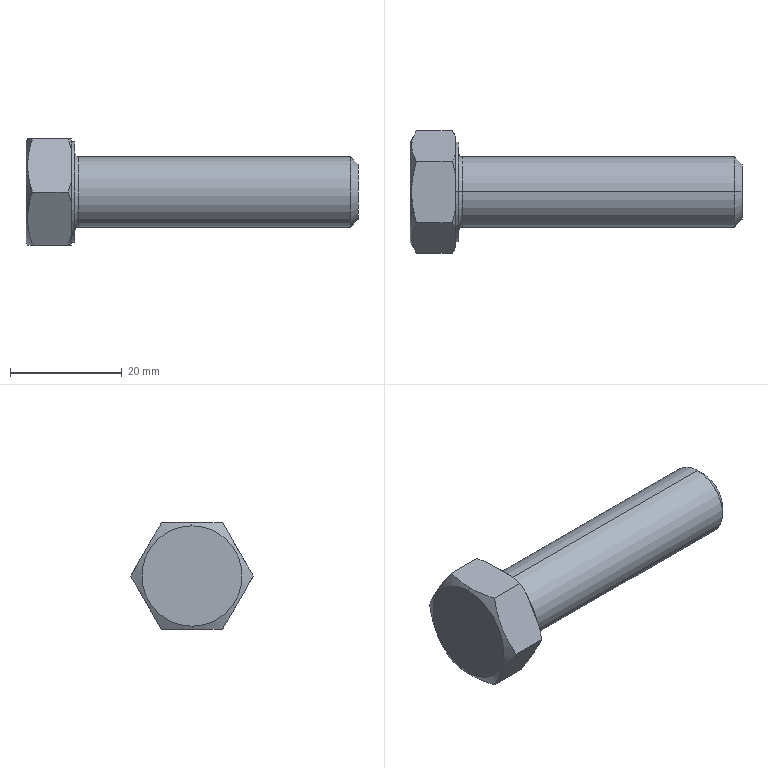Part | SolidWorks | features RevCut 4, Chamfer 1, Extrusion 1, Fillet 1, LPattern 1, Revolution 1 | 1 solid | 26 faces | box 59.531 x 21.997 x 19.05 mm | volume 9087 mm3 | cone 10 | plane 10 | cylinder 4 | torus 2 | commonest cylinder face diameters 12.7 x2 18 x2
STEP:
#1=CARTESIAN_POINT('',(9.331,0.,6.35));
#2=VERTEX_POINT('',#1);
#3=CARTESIAN_POINT('',(9.331,0.,-6.35));
#4=VERTEX_POINT('',#3);
#5=CARTESIAN_POINT('',(9.331,0.,0.));
#6=DIRECTION('',(1.,0.,0.));
#7=DIRECTION('',(0.,0.,-1.));
#8=AXIS2_PLACEMENT_3D('',#5,#6,#7);
#9=CIRCLE('',#8,6.35);
#10=EDGE_CURVE('',#2,#4,#9,.T.);
#11=ORIENTED_EDGE('',*,*,#10,.F.);
#12=CARTESIAN_POINT('',(8.731,0.,6.95));
#13=VERTEX_POINT('',#12);
#14=CARTESIAN_POINT('',(9.331,0.,6.95));
#15=DIRECTION('',(0.,1.,0.));
#16=DIRECTION('',(0.,0.,1.));
#17=AXIS2_PLACEMENT_3D('',#14,#15,#16);
#18=CIRCLE('',#17,0.6);
#19=EDGE_CURVE('',#2,#13,#18,.T.);
#20=ORIENTED_EDGE('',*,*,#19,.T.);
#21=CARTESIAN_POINT('',(8.731,0.,-6.95));
#22=VERTEX_POINT('',#21);
#23=CARTESIAN_POINT('',(8.731,0.,0.));
#24=DIRECTION('',(-1.,0.,0.));
#25=DIRECTION('',(0.,0.,-1.));
#26=AXIS2_PLACEMENT_3D('',#23,#24,#25);
#27=CIRCLE('',#26,6.95);
#28=EDGE_CURVE('',#22,#13,#27,.T.);
#29=ORIENTED_EDGE('',*,*,#28,.F.);
#30=CARTESIAN_POINT('',(9.331,0.,-6.95));
#31=DIRECTION('',(0.,-1.,0.));
#32=DIRECTION('',(0.,0.,-1.));
#33=AXIS2_PLACEMENT_3D('',#30,#31,#32);
#34=CIRCLE('',#33,0.6);
#35=EDGE_CURVE('',#4,#22,#34,.T.);
#36=ORIENTED_EDGE('',*,*,#35,.F.);
#37=EDGE_LOOP('',(#11,#20,#29,#36));
#38=FACE_OUTER_BOUND('',#37,.T.);
#39=CARTESIAN_POINT('',(9.331,0.,0.));
#40=DIRECTION('',(1.,0.,0.));
#41=DIRECTION('',(0.,0.,-1.));
#42=AXIS2_PLACEMENT_3D('',#39,#40,#41);
#43=TOROIDAL_SURFACE('',#42,6.95,0.6);
#44=ADVANCED_FACE('',(#38),#43,.F.);
#45=CARTESIAN_POINT('',(59.531,0.,-4.95));
#46=VERTEX_POINT('',#45);
#47=CARTESIAN_POINT('',(59.531,0.,4.95));
#48=VERTEX_POINT('',#47);
#49=CARTESIAN_POINT('',(59.531,0.,0.));
#50=DIRECTION('',(1.,0.,0.));
#51=DIRECTION('',(0.,0.,1.));
#52=AXIS2_PLACEMENT_3D('',#49,#50,#51);
#53=CIRCLE('',#52,4.95);
#54=EDGE_CURVE('',#46,#48,#53,.T.);
#55=ORIENTED_EDGE('',*,*,#54,.F.);
#56=CARTESIAN_POINT('',(58.131,0.,-6.35));
#57=VERTEX_POINT('',#56);
#58=CARTESIAN_POINT('',(58.131,0.,-6.35));
#59=DIRECTION('',(-0.7071,0.,-0.7071));
#60=VECTOR('',#59,1000.);
#61=LINE('',#58,#60);
#62=EDGE_CURVE('',#46,#57,#61,.T.);
#63=ORIENTED_EDGE('',*,*,#62,.T.);
#64=CARTESIAN_POINT('',(58.131,0.,6.35));
#65=VERTEX_POINT('',#64);
#66=CARTESIAN_POINT('',(58.131,0.,0.));
#67=DIRECTION('',(-1.,0.,0.));
#68=DIRECTION('',(0.,0.,1.));
#69=AXIS2_PLACEMENT_3D('',#66,#67,#68);
#70=CIRCLE('',#69,6.35);
#71=EDGE_CURVE('',#65,#57,#70,.T.);
#72=ORIENTED_EDGE('',*,*,#71,.F.);
#73=CARTESIAN_POINT('',(58.131,0.,6.35));
#74=DIRECTION('',(-0.7071,0.,0.7071));
#75=VECTOR('',#74,1000.);
#76=LINE('',#73,#75);
#77=EDGE_CURVE('',#48,#65,#76,.T.);
#78=ORIENTED_EDGE('',*,*,#77,.F.);
#79=EDGE_LOOP('',(#55,#63,#72,#78));
#80=FACE_OUTER_BOUND('',#79,.T.);
#81=CARTESIAN_POINT('',(58.131,0.,0.));
#82=DIRECTION('',(-1.,0.,0.));
#83=DIRECTION('',(0.,0.,1.));
#84=AXIS2_PLACEMENT_3D('',#81,#82,#83);
#85=CONICAL_SURFACE('',#84,6.35,0.7854);
#86=ADVANCED_FACE('',(#80),#85,.T.);
#87=ORIENTED_EDGE('',*,*,#71,.T.);
#88=CARTESIAN_POINT('',(0.,0.,-6.35));
#89=DIRECTION('',(-1.,0.,0.));
#90=VECTOR('',#89,1000.);
#91=LINE('',#88,#90);
#92=EDGE_CURVE('',#57,#4,#91,.T.);
#93=ORIENTED_EDGE('',*,*,#92,.T.);
#94=CARTESIAN_POINT('',(9.331,0.,0.));
#95=DIRECTION('',(1.,0.,0.));
#96=DIRECTION('',(0.,0.,-1.));
#97=AXIS2_PLACEMENT_3D('',#94,#95,#96);
#98=CIRCLE('',#97,6.35);
#99=EDGE_CURVE('',#4,#2,#98,.T.);
#100=ORIENTED_EDGE('',*,*,#99,.T.);
#101=CARTESIAN_POINT('',(0.,0.,6.35));
#102=DIRECTION('',(-1.,0.,0.));
#103=VECTOR('',#102,1000.);
#104=LINE('',#101,#103);
#105=EDGE_CURVE('',#65,#2,#104,.T.);
#106=ORIENTED_EDGE('',*,*,#105,.F.);
#107=EDGE_LOOP('',(#87,#93,#100,#106));
#108=FACE_OUTER_BOUND('',#107,.T.);
#109=CARTESIAN_POINT('',(0.,0.,0.));
#110=DIRECTION('',(-1.,0.,0.));
#111=DIRECTION('',(0.,0.,1.));
#112=AXIS2_PLACEMENT_3D('',#109,#110,#111);
#113=CYLINDRICAL_SURFACE('',#112,6.35);
#114=ADVANCED_FACE('',(#108),#113,.T.);
#115=CARTESIAN_POINT('',(8.731,0.,9.));
#116=VERTEX_POINT('',#115);
#117=CARTESIAN_POINT('',(8.731,0.,-9.));
#118=VERTEX_POINT('',#117);
#119=CARTESIAN_POINT('',(8.731,0.,0.));
#120=DIRECTION('',(-1.,0.,0.));
#121=DIRECTION('',(0.,0.,1.));
#122=AXIS2_PLACEMENT_3D('',#119,#120,#121);
#123=CIRCLE('',#122,9.);
#124=EDGE_CURVE('',#116,#118,#123,.T.);
#125=ORIENTED_EDGE('',*,*,#124,.T.);
#126=CARTESIAN_POINT('',(8.131,0.,-9.));
#127=VERTEX_POINT('',#126);
#128=CARTESIAN_POINT('',(0.,0.,-9.));
#129=DIRECTION('',(-1.,0.,0.));
#130=VECTOR('',#129,1000.);
#131=LINE('',#128,#130);
#132=EDGE_CURVE('',#118,#127,#131,.T.);
#133=ORIENTED_EDGE('',*,*,#132,.T.);
#134=CARTESIAN_POINT('',(8.131,0.,9.));
#135=VERTEX_POINT('',#134);
#136=CARTESIAN_POINT('',(8.131,0.,0.));
#137=DIRECTION('',(-1.,0.,0.));
#138=DIRECTION('',(0.,0.,1.));
#139=AXIS2_PLACEMENT_3D('',#136,#137,#138);
#140=CIRCLE('',#139,9.);
#141=EDGE_CURVE('',#135,#127,#140,.T.);
#142=ORIENTED_EDGE('',*,*,#141,.F.);
#143=CARTESIAN_POINT('',(0.,0.,9.));
#144=DIRECTION('',(-1.,0.,0.));
#145=VECTOR('',#144,1000.);
#146=LINE('',#143,#145);
#147=EDGE_CURVE('',#116,#135,#146,.T.);
#148=ORIENTED_EDGE('',*,*,#147,.F.);
#149=EDGE_LOOP('',(#125,#133,#142,#148));
#150=FACE_OUTER_BOUND('',#149,.T.);
#151=CARTESIAN_POINT('',(0.,0.,0.));
#152=DIRECTION('',(-1.,0.,0.));
#153=DIRECTION('',(0.,0.,1.));
#154=AXIS2_PLACEMENT_3D('',#151,#152,#153);
#155=CYLINDRICAL_SURFACE('',#154,9.);
#156=ADVANCED_FACE('',(#150),#155,.T.);
#157=CARTESIAN_POINT('',(0.,0.,9.));
#158=VERTEX_POINT('',#157);
#159=CARTESIAN_POINT('',(0.,0.,-9.));
#160=VERTEX_POINT('',#159);
#161=CARTESIAN_POINT('',(0.,0.,0.));
#162=DIRECTION('',(-1.,0.,0.));
#163=DIRECTION('',(0.,0.,1.));
#164=AXIS2_PLACEMENT_3D('',#161,#162,#163);
#165=CIRCLE('',#164,9.);
#166=EDGE_CURVE('',#158,#160,#165,.T.);
#167=ORIENTED_EDGE('',*,*,#166,.F.);
#168=CARTESIAN_POINT('',(0.3031,0.,9.525));
#169=VERTEX_POINT('',#168);
#170=CARTESIAN_POINT('',(0.,0.,9.));
#171=DIRECTION('',(0.5,0.,0.866));
#172=VECTOR('',#171,1000.);
#173=LINE('',#170,#172);
#174=EDGE_CURVE('',#158,#169,#173,.T.);
#175=ORIENTED_EDGE('',*,*,#174,.T.);
#176=CARTESIAN_POINT('',(1.154,5.499,9.525));
#177=VERTEX_POINT('',#176);
#178=CARTESIAN_POINT('',(0.3031,0.,9.525));
#179=CARTESIAN_POINT('',(0.3031,0.4656,9.525));
#180=CARTESIAN_POINT('',(0.323,0.9341,9.525));
#181=CARTESIAN_POINT('',(0.4017,1.87,9.525));
#182=CARTESIAN_POINT('',(0.4599,2.333,9.525));
#183=CARTESIAN_POINT('',(0.6834,3.709,9.525));
#184=CARTESIAN_POINT('',(0.8971,4.61,9.525));
#185=CARTESIAN_POINT('',(1.154,5.499,9.525));
#186=B_SPLINE_CURVE_WITH_KNOTS('',3,(#178,#179,#180,#181,#182,#183,#184,#185),.UNSPECIFIED.,.F.,.F.,(4,2,2,4),(0.01578,0.01717,0.01857,0.02135),.UNSPECIFIED.);
#187=EDGE_CURVE('',#169,#177,#186,.T.);
#188=ORIENTED_EDGE('',*,*,#187,.T.);
#189=CARTESIAN_POINT('',(1.154,10.999,0.));
#190=VERTEX_POINT('',#189);
#191=CARTESIAN_POINT('',(1.154,5.499,9.525));
#192=CARTESIAN_POINT('',(0.8946,5.948,8.747));
#193=CARTESIAN_POINT('',(0.681,6.4,7.964));
#194=CARTESIAN_POINT('',(0.3851,7.314,6.381));
#195=CARTESIAN_POINT('',(0.3037,7.776,5.581));
#196=CARTESIAN_POINT('',(0.3028,8.477,4.367));
#197=CARTESIAN_POINT('',(0.3227,8.712,3.96));
#198=CARTESIAN_POINT('',(0.4002,9.177,3.155));
#199=CARTESIAN_POINT('',(0.4578,9.408,2.756));
#200=CARTESIAN_POINT('',(0.6802,10.096,1.564));
#201=CARTESIAN_POINT('',(0.8943,10.549,0.7786));
#202=CARTESIAN_POINT('',(1.154,10.999,0.));
#203=B_SPLINE_CURVE_WITH_KNOTS('',3,(#191,#192,#193,#194,#195,#196,#197,#198,#199,#200,#201,#202),.UNSPECIFIED.,.F.,.F.,(4,2,2,2,2,4),(0.000000238,0.002777,0.005554,0.006943,0.008331,0.01111),.UNSPECIFIED.);
#204=EDGE_CURVE('',#177,#190,#203,.T.);
#205=ORIENTED_EDGE('',*,*,#204,.T.);
#206=CARTESIAN_POINT('',(1.154,5.499,-9.525));
#207=VERTEX_POINT('',#206);
#208=CARTESIAN_POINT('',(1.154,10.999,0.));
#209=CARTESIAN_POINT('',(0.8946,10.55,-0.7776));
#210=CARTESIAN_POINT('',(0.681,10.097,-1.561));
#211=CARTESIAN_POINT('',(0.3851,9.183,-3.144));
#212=CARTESIAN_POINT('',(0.3037,8.722,-3.944));
#213=CARTESIAN_POINT('',(0.3028,8.02,-5.158));
#214=CARTESIAN_POINT('',(0.3227,7.786,-5.565));
#215=CARTESIAN_POINT('',(0.4002,7.321,-6.37));
#216=CARTESIAN_POINT('',(0.4578,7.09,-6.769));
#217=CARTESIAN_POINT('',(0.6802,6.402,-7.961));
#218=CARTESIAN_POINT('',(0.8943,5.949,-8.746));
#219=CARTESIAN_POINT('',(1.154,5.499,-9.525));
#220=B_SPLINE_CURVE_WITH_KNOTS('',3,(#208,#209,#210,#211,#212,#213,#214,#215,#216,#217,#218,#219),.UNSPECIFIED.,.F.,.F.,(4,2,2,2,2,4),(0.000000238,0.002777,0.005554,0.006943,0.008331,0.01111),.UNSPECIFIED.);
#221=EDGE_CURVE('',#190,#207,#220,.T.);
#222=ORIENTED_EDGE('',*,*,#221,.T.);
#223=CARTESIAN_POINT('',(0.3031,0.,-9.525));
#224=VERTEX_POINT('',#223);
#225=CARTESIAN_POINT('',(1.154,5.499,-9.525));
#226=CARTESIAN_POINT('',(0.8971,4.61,-9.525));
#227=CARTESIAN_POINT('',(0.6834,3.709,-9.525));
#228=CARTESIAN_POINT('',(0.4599,2.333,-9.525));
#229=CARTESIAN_POINT('',(0.4017,1.87,-9.525));
#230=CARTESIAN_POINT('',(0.323,0.9341,-9.525));
#231=CARTESIAN_POINT('',(0.3031,0.4656,-9.525));
#232=CARTESIAN_POINT('',(0.3031,0.,-9.525));
#233=B_SPLINE_CURVE_WITH_KNOTS('',3,(#225,#226,#227,#228,#229,#230,#231,#232),.UNSPECIFIED.,.F.,.F.,(4,2,2,4),(0.02694,0.02972,0.03112,0.03251),.UNSPECIFIED.);
#234=EDGE_CURVE('',#207,#224,#233,.T.);
#235=ORIENTED_EDGE('',*,*,#234,.T.);
#236=CARTESIAN_POINT('',(0.,0.,-9.));
#237=DIRECTION('',(0.5,0.,-0.866));
#238=VECTOR('',#237,1000.);
#239=LINE('',#236,#238);
#240=EDGE_CURVE('',#160,#224,#239,.T.);
#241=ORIENTED_EDGE('',*,*,#240,.F.);
#242=EDGE_LOOP('',(#167,#175,#188,#205,#222,#235,#241));
#243=FACE_OUTER_BOUND('',#242,.T.);
#244=CARTESIAN_POINT('',(0.,0.,0.));
#245=DIRECTION('',(1.,0.,0.));
#246=DIRECTION('',(0.,0.,-1.));
#247=AXIS2_PLACEMENT_3D('',#244,#245,#246);
#248=CONICAL_SURFACE('',#247,9.,1.047);
#249=ADVANCED_FACE('',(#243),#248,.T.);
#250=CARTESIAN_POINT('',(8.131,6.663,-7.509));
#251=VERTEX_POINT('',#250);
#252=CARTESIAN_POINT('',(8.131,9.835,-2.016));
#253=VERTEX_POINT('',#252);
#254=CARTESIAN_POINT('',(8.131,5.499,-9.525));
#255=DIRECTION('',(0.,0.5,0.866));
#256=VECTOR('',#255,1000.);
#257=LINE('',#254,#256);
#258=EDGE_CURVE('',#251,#253,#257,.T.);
#259=ORIENTED_EDGE('',*,*,#258,.F.);
#260=CARTESIAN_POINT('',(7.577,5.499,-9.525));
#261=VERTEX_POINT('',#260);
#262=CARTESIAN_POINT('',(7.577,5.499,-9.525));
#263=CARTESIAN_POINT('',(7.8,5.884,-8.858));
#264=CARTESIAN_POINT('',(7.989,6.272,-8.186));
#265=CARTESIAN_POINT('',(8.131,6.663,-7.509));
#266=B_SPLINE_CURVE_WITH_KNOTS('',3,(#262,#263,#264,#265),.UNSPECIFIED.,.F.,.F.,(4,4),(0.000000238,0.002383),.UNSPECIFIED.);
#267=EDGE_CURVE('',#261,#251,#266,.T.);
#268=ORIENTED_EDGE('',*,*,#267,.F.);
#269=CARTESIAN_POINT('',(8.731,5.499,-9.525));
#270=DIRECTION('',(-1.,0.,0.));
#271=VECTOR('',#270,1000.);
#272=LINE('',#269,#271);
#273=EDGE_CURVE('',#261,#207,#272,.T.);
#274=ORIENTED_EDGE('',*,*,#273,.T.);
#275=ORIENTED_EDGE('',*,*,#221,.F.);
#276=CARTESIAN_POINT('',(7.577,10.999,0.));
#277=VERTEX_POINT('',#276);
#278=CARTESIAN_POINT('',(8.731,10.999,0.));
#279=DIRECTION('',(-1.,0.,0.));
#280=VECTOR('',#279,1000.);
#281=LINE('',#278,#280);
#282=EDGE_CURVE('',#277,#190,#281,.T.);
#283=ORIENTED_EDGE('',*,*,#282,.F.);
#284=CARTESIAN_POINT('',(8.131,9.835,-2.016));
#285=CARTESIAN_POINT('',(7.988,10.226,-1.338));
#286=CARTESIAN_POINT('',(7.8,10.614,-0.6665));
#287=CARTESIAN_POINT('',(7.577,10.999,0.));
#288=B_SPLINE_CURVE_WITH_KNOTS('',3,(#284,#285,#286,#287),.UNSPECIFIED.,.F.,.F.,(4,4),(0.008731,0.01111),.UNSPECIFIED.);
#289=EDGE_CURVE('',#253,#277,#288,.T.);
#290=ORIENTED_EDGE('',*,*,#289,.F.);
#291=EDGE_LOOP('',(#259,#268,#274,#275,#283,#290));
#292=FACE_OUTER_BOUND('',#291,.T.);
#293=CARTESIAN_POINT('',(8.731,5.499,-9.525));
#294=DIRECTION('',(0.,-0.866,0.5));
#295=DIRECTION('',(0.,-0.5,-0.866));
#296=AXIS2_PLACEMENT_3D('',#293,#294,#295);
#297=PLANE('',#296);
#298=ADVANCED_FACE('',(#292),#297,.F.);
#299=CARTESIAN_POINT('',(8.131,9.835,2.016));
#300=VERTEX_POINT('',#299);
#301=CARTESIAN_POINT('',(8.131,6.663,7.509));
#302=VERTEX_POINT('',#301);
#303=CARTESIAN_POINT('',(8.131,10.999,0.));
#304=DIRECTION('',(0.,-0.5,0.866));
#305=VECTOR('',#304,1000.);
#306=LINE('',#303,#305);
#307=EDGE_CURVE('',#300,#302,#306,.T.);
#308=ORIENTED_EDGE('',*,*,#307,.F.);
#309=CARTESIAN_POINT('',(7.577,10.999,0.));
#310=CARTESIAN_POINT('',(7.8,10.613,0.6672));
#311=CARTESIAN_POINT('',(7.989,10.226,1.339));
#312=CARTESIAN_POINT('',(8.131,9.835,2.016));
#313=B_SPLINE_CURVE_WITH_KNOTS('',3,(#309,#310,#311,#312),.UNSPECIFIED.,.F.,.F.,(4,4),(0.000000238,0.002383),.UNSPECIFIED.);
#314=EDGE_CURVE('',#277,#300,#313,.T.);
#315=ORIENTED_EDGE('',*,*,#314,.F.);
#316=ORIENTED_EDGE('',*,*,#282,.T.);
#317=ORIENTED_EDGE('',*,*,#204,.F.);
#318=CARTESIAN_POINT('',(7.577,5.499,9.525));
#319=VERTEX_POINT('',#318);
#320=CARTESIAN_POINT('',(8.731,5.499,9.525));
#321=DIRECTION('',(-1.,0.,0.));
#322=VECTOR('',#321,1000.);
#323=LINE('',#320,#322);
#324=EDGE_CURVE('',#319,#177,#323,.T.);
#325=ORIENTED_EDGE('',*,*,#324,.F.);
#326=CARTESIAN_POINT('',(8.131,6.663,7.509));
#327=CARTESIAN_POINT('',(7.988,6.272,8.187));
#328=CARTESIAN_POINT('',(7.8,5.884,8.859));
#329=CARTESIAN_POINT('',(7.577,5.499,9.525));
#330=B_SPLINE_CURVE_WITH_KNOTS('',3,(#326,#327,#328,#329),.UNSPECIFIED.,.F.,.F.,(4,4),(0.008731,0.01111),.UNSPECIFIED.);
#331=EDGE_CURVE('',#302,#319,#330,.T.);
#332=ORIENTED_EDGE('',*,*,#331,.F.);
#333=EDGE_LOOP('',(#308,#315,#316,#317,#325,#332));
#334=FACE_OUTER_BOUND('',#333,.T.);
#335=CARTESIAN_POINT('',(8.731,10.999,0.));
#336=DIRECTION('',(0.,-0.866,-0.5));
#337=DIRECTION('',(0.,0.5,-0.866));
#338=AXIS2_PLACEMENT_3D('',#335,#336,#337);
#339=PLANE('',#338);
#340=ADVANCED_FACE('',(#334),#339,.F.);
#341=CARTESIAN_POINT('',(8.131,3.172,9.525));
#342=VERTEX_POINT('',#341);
#343=CARTESIAN_POINT('',(8.131,-3.172,9.525));
#344=VERTEX_POINT('',#343);
#345=CARTESIAN_POINT('',(8.131,5.499,9.525));
#346=DIRECTION('',(0.,-1.,0.));
#347=VECTOR('',#346,1000.);
#348=LINE('',#345,#347);
#349=EDGE_CURVE('',#342,#344,#348,.T.);
#350=ORIENTED_EDGE('',*,*,#349,.F.);
#351=CARTESIAN_POINT('',(7.577,5.499,9.525));
#352=CARTESIAN_POINT('',(7.799,4.733,9.525));
#353=CARTESIAN_POINT('',(7.988,3.958,9.525));
#354=CARTESIAN_POINT('',(8.131,3.172,9.525));
#355=B_SPLINE_CURVE_WITH_KNOTS('',3,(#351,#352,#353,#354),.UNSPECIFIED.,.F.,.F.,(4,4),(0.02694,0.02934),.UNSPECIFIED.);
#356=EDGE_CURVE('',#319,#342,#355,.T.);
#357=ORIENTED_EDGE('',*,*,#356,.F.);
#358=ORIENTED_EDGE('',*,*,#324,.T.);
#359=ORIENTED_EDGE('',*,*,#187,.F.);
#360=CARTESIAN_POINT('',(1.154,-5.499,9.525));
#361=VERTEX_POINT('',#360);
#362=CARTESIAN_POINT('',(1.154,-5.499,9.525));
#363=CARTESIAN_POINT('',(0.8953,-4.604,9.525));
#364=CARTESIAN_POINT('',(0.679,-3.688,9.525));
#365=CARTESIAN_POINT('',(0.3832,-1.854,9.525));
#366=CARTESIAN_POINT('',(0.3031,-0.9305,9.525));
#367=CARTESIAN_POINT('',(0.3031,0.,9.525));
#368=B_SPLINE_CURVE_WITH_KNOTS('',3,(#362,#363,#364,#365,#366,#367),.UNSPECIFIED.,.F.,.F.,(4,2,4),(0.01021,0.013,0.01578),.UNSPECIFIED.);
#369=EDGE_CURVE('',#361,#169,#368,.T.);
#370=ORIENTED_EDGE('',*,*,#369,.F.);
#371=CARTESIAN_POINT('',(7.577,-5.499,9.525));
#372=VERTEX_POINT('',#371);
#373=CARTESIAN_POINT('',(8.731,-5.499,9.525));
#374=DIRECTION('',(-1.,0.,0.));
#375=VECTOR('',#374,1000.);
#376=LINE('',#373,#375);
#377=EDGE_CURVE('',#372,#361,#376,.T.);
#378=ORIENTED_EDGE('',*,*,#377,.F.);
#379=CARTESIAN_POINT('',(8.131,-3.172,9.525));
#380=CARTESIAN_POINT('',(7.989,-3.954,9.525));
#381=CARTESIAN_POINT('',(7.798,-4.734,9.525));
#382=CARTESIAN_POINT('',(7.577,-5.499,9.525));
#383=B_SPLINE_CURVE_WITH_KNOTS('',3,(#379,#380,#381,#382),.UNSPECIFIED.,.F.,.F.,(4,4),(0.0357,0.03808),.UNSPECIFIED.);
#384=EDGE_CURVE('',#344,#372,#383,.T.);
#385=ORIENTED_EDGE('',*,*,#384,.F.);
#386=EDGE_LOOP('',(#350,#357,#358,#359,#370,#378,#385));
#387=FACE_OUTER_BOUND('',#386,.T.);
#388=CARTESIAN_POINT('',(8.731,5.499,9.525));
#389=DIRECTION('',(0.,0.,-1.));
#390=DIRECTION('',(-1.,0.,0.));
#391=AXIS2_PLACEMENT_3D('',#388,#389,#390);
#392=PLANE('',#391);
#393=ADVANCED_FACE('',(#387),#392,.F.);
#394=CARTESIAN_POINT('',(8.131,-6.663,7.509));
#395=VERTEX_POINT('',#394);
#396=CARTESIAN_POINT('',(8.131,-9.835,2.016));
#397=VERTEX_POINT('',#396);
#398=CARTESIAN_POINT('',(8.131,-10.999,0.));
#399=DIRECTION('',(0.,-0.5,-0.866));
#400=VECTOR('',#399,1000.);
#401=LINE('',#398,#400);
#402=EDGE_CURVE('',#395,#397,#401,.T.);
#403=ORIENTED_EDGE('',*,*,#402,.F.);
#404=CARTESIAN_POINT('',(7.577,-5.499,9.525));
#405=CARTESIAN_POINT('',(7.8,-5.884,8.858));
#406=CARTESIAN_POINT('',(7.989,-6.272,8.186));
#407=CARTESIAN_POINT('',(8.131,-6.663,7.509));
#408=B_SPLINE_CURVE_WITH_KNOTS('',3,(#404,#405,#406,#407),.UNSPECIFIED.,.F.,.F.,(4,4),(0.000000238,0.002383),.UNSPECIFIED.);
#409=EDGE_CURVE('',#372,#395,#408,.T.);
#410=ORIENTED_EDGE('',*,*,#409,.F.);
#411=ORIENTED_EDGE('',*,*,#377,.T.);
#412=CARTESIAN_POINT('',(1.154,-10.999,0.));
#413=VERTEX_POINT('',#412);
#414=CARTESIAN_POINT('',(1.154,-10.999,0.));
#415=CARTESIAN_POINT('',(0.8946,-10.55,0.7776));
#416=CARTESIAN_POINT('',(0.681,-10.097,1.561));
#417=CARTESIAN_POINT('',(0.3851,-9.183,3.144));
#418=CARTESIAN_POINT('',(0.3037,-8.722,3.944));
#419=CARTESIAN_POINT('',(0.3028,-8.02,5.158));
#420=CARTESIAN_POINT('',(0.3227,-7.786,5.565));
#421=CARTESIAN_POINT('',(0.4002,-7.321,6.37));
#422=CARTESIAN_POINT('',(0.4578,-7.09,6.769));
#423=CARTESIAN_POINT('',(0.6802,-6.402,7.961));
#424=CARTESIAN_POINT('',(0.8943,-5.949,8.746));
#425=CARTESIAN_POINT('',(1.154,-5.499,9.525));
#426=B_SPLINE_CURVE_WITH_KNOTS('',3,(#414,#415,#416,#417,#418,#419,#420,#421,#422,#423,#424,#425),.UNSPECIFIED.,.F.,.F.,(4,2,2,2,2,4),(0.000000238,0.002777,0.005554,0.006943,0.008331,0.01111),.UNSPECIFIED.);
#427=EDGE_CURVE('',#413,#361,#426,.T.);
#428=ORIENTED_EDGE('',*,*,#427,.F.);
#429=CARTESIAN_POINT('',(7.577,-10.999,0.));
#430=VERTEX_POINT('',#429);
#431=CARTESIAN_POINT('',(8.731,-10.999,0.));
#432=DIRECTION('',(-1.,0.,0.));
#433=VECTOR('',#432,1000.);
#434=LINE('',#431,#433);
#435=EDGE_CURVE('',#430,#413,#434,.T.);
#436=ORIENTED_EDGE('',*,*,#435,.F.);
#437=CARTESIAN_POINT('',(8.131,-9.835,2.016));
#438=CARTESIAN_POINT('',(7.988,-10.226,1.338));
#439=CARTESIAN_POINT('',(7.8,-10.614,0.6665));
#440=CARTESIAN_POINT('',(7.577,-10.999,0.));
#441=B_SPLINE_CURVE_WITH_KNOTS('',3,(#437,#438,#439,#440),.UNSPECIFIED.,.F.,.F.,(4,4),(0.008731,0.01111),.UNSPECIFIED.);
#442=EDGE_CURVE('',#397,#430,#441,.T.);
#443=ORIENTED_EDGE('',*,*,#442,.F.);
#444=EDGE_LOOP('',(#403,#410,#411,#428,#436,#443));
#445=FACE_OUTER_BOUND('',#444,.T.);
#446=CARTESIAN_POINT('',(8.731,-10.999,0.));
#447=DIRECTION('',(0.,0.866,-0.5));
#448=DIRECTION('',(0.,0.5,0.866));
#449=AXIS2_PLACEMENT_3D('',#446,#447,#448);
#450=PLANE('',#449);
#451=ADVANCED_FACE('',(#445),#450,.F.);
#452=CARTESIAN_POINT('',(8.131,-9.835,-2.016));
#453=VERTEX_POINT('',#452);
#454=CARTESIAN_POINT('',(8.131,-6.663,-7.509));
#455=VERTEX_POINT('',#454);
#456=CARTESIAN_POINT('',(8.131,-5.499,-9.525));
#457=DIRECTION('',(0.,0.5,-0.866));
#458=VECTOR('',#457,1000.);
#459=LINE('',#456,#458);
#460=EDGE_CURVE('',#453,#455,#459,.T.);
#461=ORIENTED_EDGE('',*,*,#460,.F.);
#462=CARTESIAN_POINT('',(7.577,-10.999,0.));
#463=CARTESIAN_POINT('',(7.8,-10.613,-0.6672));
#464=CARTESIAN_POINT('',(7.989,-10.226,-1.339));
#465=CARTESIAN_POINT('',(8.131,-9.835,-2.016));
#466=B_SPLINE_CURVE_WITH_KNOTS('',3,(#462,#463,#464,#465),.UNSPECIFIED.,.F.,.F.,(4,4),(0.000000238,0.002383),.UNSPECIFIED.);
#467=EDGE_CURVE('',#430,#453,#466,.T.);
#468=ORIENTED_EDGE('',*,*,#467,.F.);
#469=ORIENTED_EDGE('',*,*,#435,.T.);
#470=CARTESIAN_POINT('',(1.154,-5.499,-9.525));
#471=VERTEX_POINT('',#470);
#472=CARTESIAN_POINT('',(1.154,-5.499,-9.525));
#473=CARTESIAN_POINT('',(0.8946,-5.948,-8.747));
#474=CARTESIAN_POINT('',(0.681,-6.4,-7.964));
#475=CARTESIAN_POINT('',(0.3851,-7.314,-6.381));
#476=CARTESIAN_POINT('',(0.3037,-7.776,-5.581));
#477=CARTESIAN_POINT('',(0.3028,-8.477,-4.367));
#478=CARTESIAN_POINT('',(0.3227,-8.712,-3.96));
#479=CARTESIAN_POINT('',(0.4002,-9.177,-3.155));
#480=CARTESIAN_POINT('',(0.4578,-9.408,-2.756));
#481=CARTESIAN_POINT('',(0.6802,-10.096,-1.564));
#482=CARTESIAN_POINT('',(0.8943,-10.549,-0.7786));
#483=CARTESIAN_POINT('',(1.154,-10.999,0.));
#484=B_SPLINE_CURVE_WITH_KNOTS('',3,(#472,#473,#474,#475,#476,#477,#478,#479,#480,#481,#482,#483),.UNSPECIFIED.,.F.,.F.,(4,2,2,2,2,4),(0.000000238,0.002777,0.005554,0.006943,0.008331,0.01111),.UNSPECIFIED.);
#485=EDGE_CURVE('',#471,#413,#484,.T.);
#486=ORIENTED_EDGE('',*,*,#485,.F.);
#487=CARTESIAN_POINT('',(7.577,-5.499,-9.525));
#488=VERTEX_POINT('',#487);
#489=CARTESIAN_POINT('',(8.731,-5.499,-9.525));
#490=DIRECTION('',(-1.,0.,0.));
#491=VECTOR('',#490,1000.);
#492=LINE('',#489,#491);
#493=EDGE_CURVE('',#488,#471,#492,.T.);
#494=ORIENTED_EDGE('',*,*,#493,.F.);
#495=CARTESIAN_POINT('',(8.131,-6.663,-7.509));
#496=CARTESIAN_POINT('',(7.988,-6.272,-8.187));
#497=CARTESIAN_POINT('',(7.8,-5.884,-8.859));
#498=CARTESIAN_POINT('',(7.577,-5.499,-9.525));
#499=B_SPLINE_CURVE_WITH_KNOTS('',3,(#495,#496,#497,#498),.UNSPECIFIED.,.F.,.F.,(4,4),(0.008731,0.01111),.UNSPECIFIED.);
#500=EDGE_CURVE('',#455,#488,#499,.T.);
#501=ORIENTED_EDGE('',*,*,#500,.F.);
#502=EDGE_LOOP('',(#461,#468,#469,#486,#494,#501));
#503=FACE_OUTER_BOUND('',#502,.T.);
#504=CARTESIAN_POINT('',(8.731,-5.499,-9.525));
#505=DIRECTION('',(0.,0.866,0.5));
#506=DIRECTION('',(0.,-0.5,0.866));
#507=AXIS2_PLACEMENT_3D('',#504,#505,#506);
#508=PLANE('',#507);
#509=ADVANCED_FACE('',(#503),#508,.F.);
#510=CARTESIAN_POINT('',(8.131,-3.172,-9.525));
#511=VERTEX_POINT('',#510);
#512=CARTESIAN_POINT('',(8.131,3.172,-9.525));
#513=VERTEX_POINT('',#512);
#514=CARTESIAN_POINT('',(8.131,5.499,-9.525));
#515=DIRECTION('',(0.,1.,0.));
#516=VECTOR('',#515,1000.);
#517=LINE('',#514,#516);
#518=EDGE_CURVE('',#511,#513,#517,.T.);
#519=ORIENTED_EDGE('',*,*,#518,.F.);
#520=CARTESIAN_POINT('',(7.577,-5.499,-9.525));
#521=CARTESIAN_POINT('',(7.798,-4.734,-9.525));
#522=CARTESIAN_POINT('',(7.989,-3.954,-9.525));
#523=CARTESIAN_POINT('',(8.131,-3.172,-9.525));
#524=B_SPLINE_CURVE_WITH_KNOTS('',3,(#520,#521,#522,#523),.UNSPECIFIED.,.F.,.F.,(4,4),(0.01021,0.01259),.UNSPECIFIED.);
#525=EDGE_CURVE('',#488,#511,#524,.T.);
#526=ORIENTED_EDGE('',*,*,#525,.F.);
#527=ORIENTED_EDGE('',*,*,#493,.T.);
#528=CARTESIAN_POINT('',(0.3031,0.,-9.525));
#529=CARTESIAN_POINT('',(0.3031,-0.9305,-9.525));
#530=CARTESIAN_POINT('',(0.3832,-1.854,-9.525));
#531=CARTESIAN_POINT('',(0.679,-3.688,-9.525));
#532=CARTESIAN_POINT('',(0.8953,-4.604,-9.525));
#533=CARTESIAN_POINT('',(1.154,-5.499,-9.525));
#534=B_SPLINE_CURVE_WITH_KNOTS('',3,(#528,#529,#530,#531,#532,#533),.UNSPECIFIED.,.F.,.F.,(4,2,4),(0.03251,0.03529,0.03808),.UNSPECIFIED.);
#535=EDGE_CURVE('',#224,#471,#534,.T.);
#536=ORIENTED_EDGE('',*,*,#535,.F.);
#537=ORIENTED_EDGE('',*,*,#234,.F.);
#538=ORIENTED_EDGE('',*,*,#273,.F.);
#539=CARTESIAN_POINT('',(8.131,3.172,-9.525));
#540=CARTESIAN_POINT('',(7.988,3.958,-9.525));
#541=CARTESIAN_POINT('',(7.799,4.733,-9.525));
#542=CARTESIAN_POINT('',(7.577,5.499,-9.525));
#543=B_SPLINE_CURVE_WITH_KNOTS('',3,(#539,#540,#541,#542),.UNSPECIFIED.,.F.,.F.,(4,4),(0.01895,0.02135),.UNSPECIFIED.);
#544=EDGE_CURVE('',#513,#261,#543,.T.);
#545=ORIENTED_EDGE('',*,*,#544,.F.);
#546=EDGE_LOOP('',(#519,#526,#527,#536,#537,#538,#545));
#547=FACE_OUTER_BOUND('',#546,.T.);
#548=CARTESIAN_POINT('',(8.731,5.499,-9.525));
#549=DIRECTION('',(0.,0.,1.));
#550=DIRECTION('',(1.,0.,0.));
#551=AXIS2_PLACEMENT_3D('',#548,#549,#550);
#552=PLANE('',#551);
#553=ADVANCED_FACE('',(#547),#552,.F.);
#554=ORIENTED_EDGE('',*,*,#525,.T.);
#555=CARTESIAN_POINT('',(8.131,0.,0.));
#556=DIRECTION('',(-1.,0.,0.));
#557=DIRECTION('',(0.,0.,-1.));
#558=AXIS2_PLACEMENT_3D('',#555,#556,#557);
#559=CIRCLE('',#558,10.039);
#560=EDGE_CURVE('',#511,#455,#559,.T.);
#561=ORIENTED_EDGE('',*,*,#560,.T.);
#562=ORIENTED_EDGE('',*,*,#500,.T.);
#563=EDGE_LOOP('',(#554,#561,#562));
#564=FACE_OUTER_BOUND('',#563,.T.);
#565=CARTESIAN_POINT('',(4.691,0.,0.));
#566=DIRECTION('',(-1.,0.,0.));
#567=DIRECTION('',(0.,0.,1.));
#568=AXIS2_PLACEMENT_3D('',#565,#566,#567);
#569=CONICAL_SURFACE('',#568,15.999,1.047);
#570=ADVANCED_FACE('',(#564),#569,.T.);
#571=ORIENTED_EDGE('',*,*,#467,.T.);
#572=CARTESIAN_POINT('',(8.131,0.,0.));
#573=DIRECTION('',(-1.,0.,0.));
#574=DIRECTION('',(0.,0.,-1.));
#575=AXIS2_PLACEMENT_3D('',#572,#573,#574);
#576=CIRCLE('',#575,10.039);
#577=EDGE_CURVE('',#453,#397,#576,.T.);
#578=ORIENTED_EDGE('',*,*,#577,.T.);
#579=ORIENTED_EDGE('',*,*,#442,.T.);
#580=EDGE_LOOP('',(#571,#578,#579));
#581=FACE_OUTER_BOUND('',#580,.T.);
#582=CARTESIAN_POINT('',(4.691,0.,0.));
#583=DIRECTION('',(-1.,0.,0.));
#584=DIRECTION('',(0.,0.,1.));
#585=AXIS2_PLACEMENT_3D('',#582,#583,#584);
#586=CONICAL_SURFACE('',#585,15.999,1.047);
#587=ADVANCED_FACE('',(#581),#586,.T.);
#588=ORIENTED_EDGE('',*,*,#409,.T.);
#589=CARTESIAN_POINT('',(8.131,0.,0.));
#590=DIRECTION('',(-1.,0.,0.));
#591=DIRECTION('',(0.,0.,-1.));
#592=AXIS2_PLACEMENT_3D('',#589,#590,#591);
#593=CIRCLE('',#592,10.039);
#594=EDGE_CURVE('',#395,#344,#593,.T.);
#595=ORIENTED_EDGE('',*,*,#594,.T.);
#596=ORIENTED_EDGE('',*,*,#384,.T.);
#597=EDGE_LOOP('',(#588,#595,#596));
#598=FACE_OUTER_BOUND('',#597,.T.);
#599=CARTESIAN_POINT('',(4.691,0.,0.));
#600=DIRECTION('',(-1.,0.,0.));
#601=DIRECTION('',(0.,0.,1.));
#602=AXIS2_PLACEMENT_3D('',#599,#600,#601);
#603=CONICAL_SURFACE('',#602,15.999,1.047);
#604=ADVANCED_FACE('',(#598),#603,.T.);
#605=ORIENTED_EDGE('',*,*,#356,.T.);
#606=CARTESIAN_POINT('',(8.131,0.,0.));
#607=DIRECTION('',(-1.,0.,0.));
#608=DIRECTION('',(0.,0.,-1.));
#609=AXIS2_PLACEMENT_3D('',#606,#607,#608);
#610=CIRCLE('',#609,10.039);
#611=EDGE_CURVE('',#342,#302,#610,.T.);
#612=ORIENTED_EDGE('',*,*,#611,.T.);
#613=ORIENTED_EDGE('',*,*,#331,.T.);
#614=EDGE_LOOP('',(#605,#612,#613));
#615=FACE_OUTER_BOUND('',#614,.T.);
#616=CARTESIAN_POINT('',(4.691,0.,0.));
#617=DIRECTION('',(-1.,0.,0.));
#618=DIRECTION('',(0.,0.,1.));
#619=AXIS2_PLACEMENT_3D('',#616,#617,#618);
#620=CONICAL_SURFACE('',#619,15.999,1.047);
#621=ADVANCED_FACE('',(#615),#620,.T.);
#622=ORIENTED_EDGE('',*,*,#314,.T.);
#623=CARTESIAN_POINT('',(8.131,0.,0.));
#624=DIRECTION('',(-1.,0.,0.));
#625=DIRECTION('',(0.,0.,-1.));
#626=AXIS2_PLACEMENT_3D('',#623,#624,#625);
#627=CIRCLE('',#626,10.039);
#628=EDGE_CURVE('',#300,#253,#627,.T.);
#629=ORIENTED_EDGE('',*,*,#628,.T.);
#630=ORIENTED_EDGE('',*,*,#289,.T.);
#631=EDGE_LOOP('',(#622,#629,#630));
#632=FACE_OUTER_BOUND('',#631,.T.);
#633=CARTESIAN_POINT('',(4.691,0.,0.));
#634=DIRECTION('',(-1.,0.,0.));
#635=DIRECTION('',(0.,0.,1.));
#636=AXIS2_PLACEMENT_3D('',#633,#634,#635);
#637=CONICAL_SURFACE('',#636,15.999,1.047);
#638=ADVANCED_FACE('',(#632),#637,.T.);
#639=ORIENTED_EDGE('',*,*,#267,.T.);
#640=CARTESIAN_POINT('',(8.131,0.,0.));
#641=DIRECTION('',(-1.,0.,0.));
#642=DIRECTION('',(0.,0.,-1.));
#643=AXIS2_PLACEMENT_3D('',#640,#641,#642);
#644=CIRCLE('',#643,10.039);
#645=EDGE_CURVE('',#251,#513,#644,.T.);
#646=ORIENTED_EDGE('',*,*,#645,.T.);
#647=ORIENTED_EDGE('',*,*,#544,.T.);
#648=EDGE_LOOP('',(#639,#646,#647));
#649=FACE_OUTER_BOUND('',#648,.T.);
#650=CARTESIAN_POINT('',(4.691,0.,0.));
#651=DIRECTION('',(-1.,0.,0.));
#652=DIRECTION('',(0.,0.,1.));
#653=AXIS2_PLACEMENT_3D('',#650,#651,#652);
#654=CONICAL_SURFACE('',#653,15.999,1.047);
#655=ADVANCED_FACE('',(#649),#654,.T.);
#656=ORIENTED_EDGE('',*,*,#174,.F.);
#657=CARTESIAN_POINT('',(0.,0.,0.));
#658=DIRECTION('',(-1.,0.,0.));
#659=DIRECTION('',(0.,0.,1.));
#660=AXIS2_PLACEMENT_3D('',#657,#658,#659);
#661=CIRCLE('',#660,9.);
#662=EDGE_CURVE('',#160,#158,#661,.T.);
#663=ORIENTED_EDGE('',*,*,#662,.F.);
#664=ORIENTED_EDGE('',*,*,#240,.T.);
#665=ORIENTED_EDGE('',*,*,#535,.T.);
#666=ORIENTED_EDGE('',*,*,#485,.T.);
#667=ORIENTED_EDGE('',*,*,#427,.T.);
#668=ORIENTED_EDGE('',*,*,#369,.T.);
#669=EDGE_LOOP('',(#656,#663,#664,#665,#666,#667,#668));
#670=FACE_OUTER_BOUND('',#669,.T.);
#671=CARTESIAN_POINT('',(0.,0.,0.));
#672=DIRECTION('',(1.,0.,0.));
#673=DIRECTION('',(0.,0.,-1.));
#674=AXIS2_PLACEMENT_3D('',#671,#672,#673);
#675=CONICAL_SURFACE('',#674,9.,1.047);
#676=ADVANCED_FACE('',(#670),#675,.T.);
#677=ORIENTED_EDGE('',*,*,#662,.T.);
#678=ORIENTED_EDGE('',*,*,#166,.T.);
#679=EDGE_LOOP('',(#677,#678));
#680=FACE_OUTER_BOUND('',#679,.T.);
#681=CARTESIAN_POINT('',(0.,10.999,0.));
#682=DIRECTION('',(1.,0.,0.));
#683=DIRECTION('',(0.,0.,-1.));
#684=AXIS2_PLACEMENT_3D('',#681,#682,#683);
#685=PLANE('',#684);
#686=ADVANCED_FACE('',(#680),#685,.F.);
#687=ORIENTED_EDGE('',*,*,#402,.T.);
#688=ORIENTED_EDGE('',*,*,#577,.F.);
#689=ORIENTED_EDGE('',*,*,#460,.T.);
#690=ORIENTED_EDGE('',*,*,#560,.F.);
#691=ORIENTED_EDGE('',*,*,#518,.T.);
#692=ORIENTED_EDGE('',*,*,#645,.F.);
#693=ORIENTED_EDGE('',*,*,#258,.T.);
#694=ORIENTED_EDGE('',*,*,#628,.F.);
#695=ORIENTED_EDGE('',*,*,#307,.T.);
#696=ORIENTED_EDGE('',*,*,#611,.F.);
#697=ORIENTED_EDGE('',*,*,#349,.T.);
#698=ORIENTED_EDGE('',*,*,#594,.F.);
#699=EDGE_LOOP('',(#687,#688,#689,#690,#691,#692,#693,#694,#695,#696,#697,#698));
#700=FACE_OUTER_BOUND('',#699,.T.);
#701=ORIENTED_EDGE('',*,*,#141,.T.);
#702=CARTESIAN_POINT('',(8.131,0.,0.));
#703=DIRECTION('',(-1.,0.,0.));
#704=DIRECTION('',(0.,0.,1.));
#705=AXIS2_PLACEMENT_3D('',#702,#703,#704);
#706=CIRCLE('',#705,9.);
#707=EDGE_CURVE('',#127,#135,#706,.T.);
#708=ORIENTED_EDGE('',*,*,#707,.T.);
#709=EDGE_LOOP('',(#701,#708));
#710=FACE_BOUND('',#709,.T.);
#711=CARTESIAN_POINT('',(8.131,9.,0.));
#712=DIRECTION('',(1.,0.,0.));
#713=DIRECTION('',(0.,0.,-1.));
#714=AXIS2_PLACEMENT_3D('',#711,#712,#713);
#715=PLANE('',#714);
#716=ADVANCED_FACE('',(#700,#710),#715,.T.);
#717=ORIENTED_EDGE('',*,*,#132,.F.);
#718=CARTESIAN_POINT('',(8.731,0.,0.));
#719=DIRECTION('',(-1.,0.,0.));
#720=DIRECTION('',(0.,0.,1.));
#721=AXIS2_PLACEMENT_3D('',#718,#719,#720);
#722=CIRCLE('',#721,9.);
#723=EDGE_CURVE('',#118,#116,#722,.T.);
#724=ORIENTED_EDGE('',*,*,#723,.T.);
#725=ORIENTED_EDGE('',*,*,#147,.T.);
#726=ORIENTED_EDGE('',*,*,#707,.F.);
#727=EDGE_LOOP('',(#717,#724,#725,#726));
#728=FACE_OUTER_BOUND('',#727,.T.);
#729=CARTESIAN_POINT('',(0.,0.,0.));
#730=DIRECTION('',(-1.,0.,0.));
#731=DIRECTION('',(0.,0.,1.));
#732=AXIS2_PLACEMENT_3D('',#729,#730,#731);
#733=CYLINDRICAL_SURFACE('',#732,9.);
#734=ADVANCED_FACE('',(#728),#733,.T.);
#735=CARTESIAN_POINT('',(59.531,0.,0.));
#736=DIRECTION('',(1.,0.,0.));
#737=DIRECTION('',(0.,0.,1.));
#738=AXIS2_PLACEMENT_3D('',#735,#736,#737);
#739=CIRCLE('',#738,4.95);
#740=EDGE_CURVE('',#48,#46,#739,.T.);
#741=ORIENTED_EDGE('',*,*,#740,.T.);
#742=ORIENTED_EDGE('',*,*,#54,.T.);
#743=EDGE_LOOP('',(#741,#742));
#744=FACE_OUTER_BOUND('',#743,.T.);
#745=CARTESIAN_POINT('',(59.531,0.,0.));
#746=DIRECTION('',(-1.,0.,0.));
#747=DIRECTION('',(0.,0.,1.));
#748=AXIS2_PLACEMENT_3D('',#745,#746,#747);
#749=PLANE('',#748);
#750=ADVANCED_FACE('',(#744),#749,.F.);
#751=ORIENTED_EDGE('',*,*,#92,.F.);
#752=CARTESIAN_POINT('',(58.131,0.,0.));
#753=DIRECTION('',(-1.,0.,0.));
#754=DIRECTION('',(0.,0.,1.));
#755=AXIS2_PLACEMENT_3D('',#752,#753,#754);
#756=CIRCLE('',#755,6.35);
#757=EDGE_CURVE('',#57,#65,#756,.T.);
#758=ORIENTED_EDGE('',*,*,#757,.T.);
#759=ORIENTED_EDGE('',*,*,#105,.T.);
#760=ORIENTED_EDGE('',*,*,#10,.T.);
#761=EDGE_LOOP('',(#751,#758,#759,#760));
#762=FACE_OUTER_BOUND('',#761,.T.);
#763=CARTESIAN_POINT('',(0.,0.,0.));
#764=DIRECTION('',(-1.,0.,0.));
#765=DIRECTION('',(0.,0.,1.));
#766=AXIS2_PLACEMENT_3D('',#763,#764,#765);
#767=CYLINDRICAL_SURFACE('',#766,6.35);
#768=ADVANCED_FACE('',(#762),#767,.T.);
#769=ORIENTED_EDGE('',*,*,#28,.T.);
#770=CARTESIAN_POINT('',(8.731,0.,0.));
#771=DIRECTION('',(-1.,0.,0.));
#772=DIRECTION('',(0.,0.,-1.));
#773=AXIS2_PLACEMENT_3D('',#770,#771,#772);
#774=CIRCLE('',#773,6.95);
#775=EDGE_CURVE('',#13,#22,#774,.T.);
#776=ORIENTED_EDGE('',*,*,#775,.T.);
#777=EDGE_LOOP('',(#769,#776));
#778=FACE_BOUND('',#777,.T.);
#779=ORIENTED_EDGE('',*,*,#124,.F.);
#780=ORIENTED_EDGE('',*,*,#723,.F.);
#781=EDGE_LOOP('',(#779,#780));
#782=FACE_OUTER_BOUND('',#781,.T.);
#783=CARTESIAN_POINT('',(8.731,10.999,0.));
#784=DIRECTION('',(1.,0.,0.));
#785=DIRECTION('',(0.,0.,-1.));
#786=AXIS2_PLACEMENT_3D('',#783,#784,#785);
#787=PLANE('',#786);
#788=ADVANCED_FACE('',(#778,#782),#787,.T.);
#789=ORIENTED_EDGE('',*,*,#62,.F.);
#790=ORIENTED_EDGE('',*,*,#740,.F.);
#791=ORIENTED_EDGE('',*,*,#77,.T.);
#792=ORIENTED_EDGE('',*,*,#757,.F.);
#793=EDGE_LOOP('',(#789,#790,#791,#792));
#794=FACE_OUTER_BOUND('',#793,.T.);
#795=CARTESIAN_POINT('',(58.131,0.,0.));
#796=DIRECTION('',(-1.,0.,0.));
#797=DIRECTION('',(0.,0.,1.));
#798=AXIS2_PLACEMENT_3D('',#795,#796,#797);
#799=CONICAL_SURFACE('',#798,6.35,0.7854);
#800=ADVANCED_FACE('',(#794),#799,.T.);
#801=ORIENTED_EDGE('',*,*,#19,.F.);
#802=ORIENTED_EDGE('',*,*,#99,.F.);
#803=ORIENTED_EDGE('',*,*,#35,.T.);
#804=ORIENTED_EDGE('',*,*,#775,.F.);
#805=EDGE_LOOP('',(#801,#802,#803,#804));
#806=FACE_OUTER_BOUND('',#805,.T.);
#807=CARTESIAN_POINT('',(9.331,0.,0.));
#808=DIRECTION('',(1.,0.,0.));
#809=DIRECTION('',(0.,0.,-1.));
#810=AXIS2_PLACEMENT_3D('',#807,#808,#809);
#811=TOROIDAL_SURFACE('',#810,6.95,0.6);
#812=ADVANCED_FACE('',(#806),#811,.F.);
#813=CLOSED_SHELL('',(#44,#86,#114,#156,#249,#298,#340,#393,#451,#509,#553,#570,#587,#604,#621,#638,#655,#676,#686,#716,#734,#750,#768,#788,#800,#812));
#814=MANIFOLD_SOLID_BREP('',#813);
#815=CARTESIAN_POINT('',(0.,0.,0.));
#816=DIRECTION('',(0.,0.,1.));
#817=DIRECTION('',(1.,0.,0.));
#818=AXIS2_PLACEMENT_3D('',#815,#816,#817);
#819=(LENGTH_UNIT()NAMED_UNIT(*)SI_UNIT(.MILLI.,.METRE.));
#820=UNCERTAINTY_MEASURE_WITH_UNIT(LENGTH_MEASURE(0.00001),#819,'','');
#821=(NAMED_UNIT(*)PLANE_ANGLE_UNIT()SI_UNIT($,.RADIAN.));
#822=(NAMED_UNIT(*)SI_UNIT($,.STERADIAN.)SOLID_ANGLE_UNIT());
#823=(GEOMETRIC_REPRESENTATION_CONTEXT(3)GLOBAL_UNCERTAINTY_ASSIGNED_CONTEXT((#820))GLOBAL_UNIT_ASSIGNED_CONTEXT((#819,#821,#822))REPRESENTATION_CONTEXT('',''));
#824=ADVANCED_BREP_SHAPE_REPRESENTATION('',(#814,#818),#823);